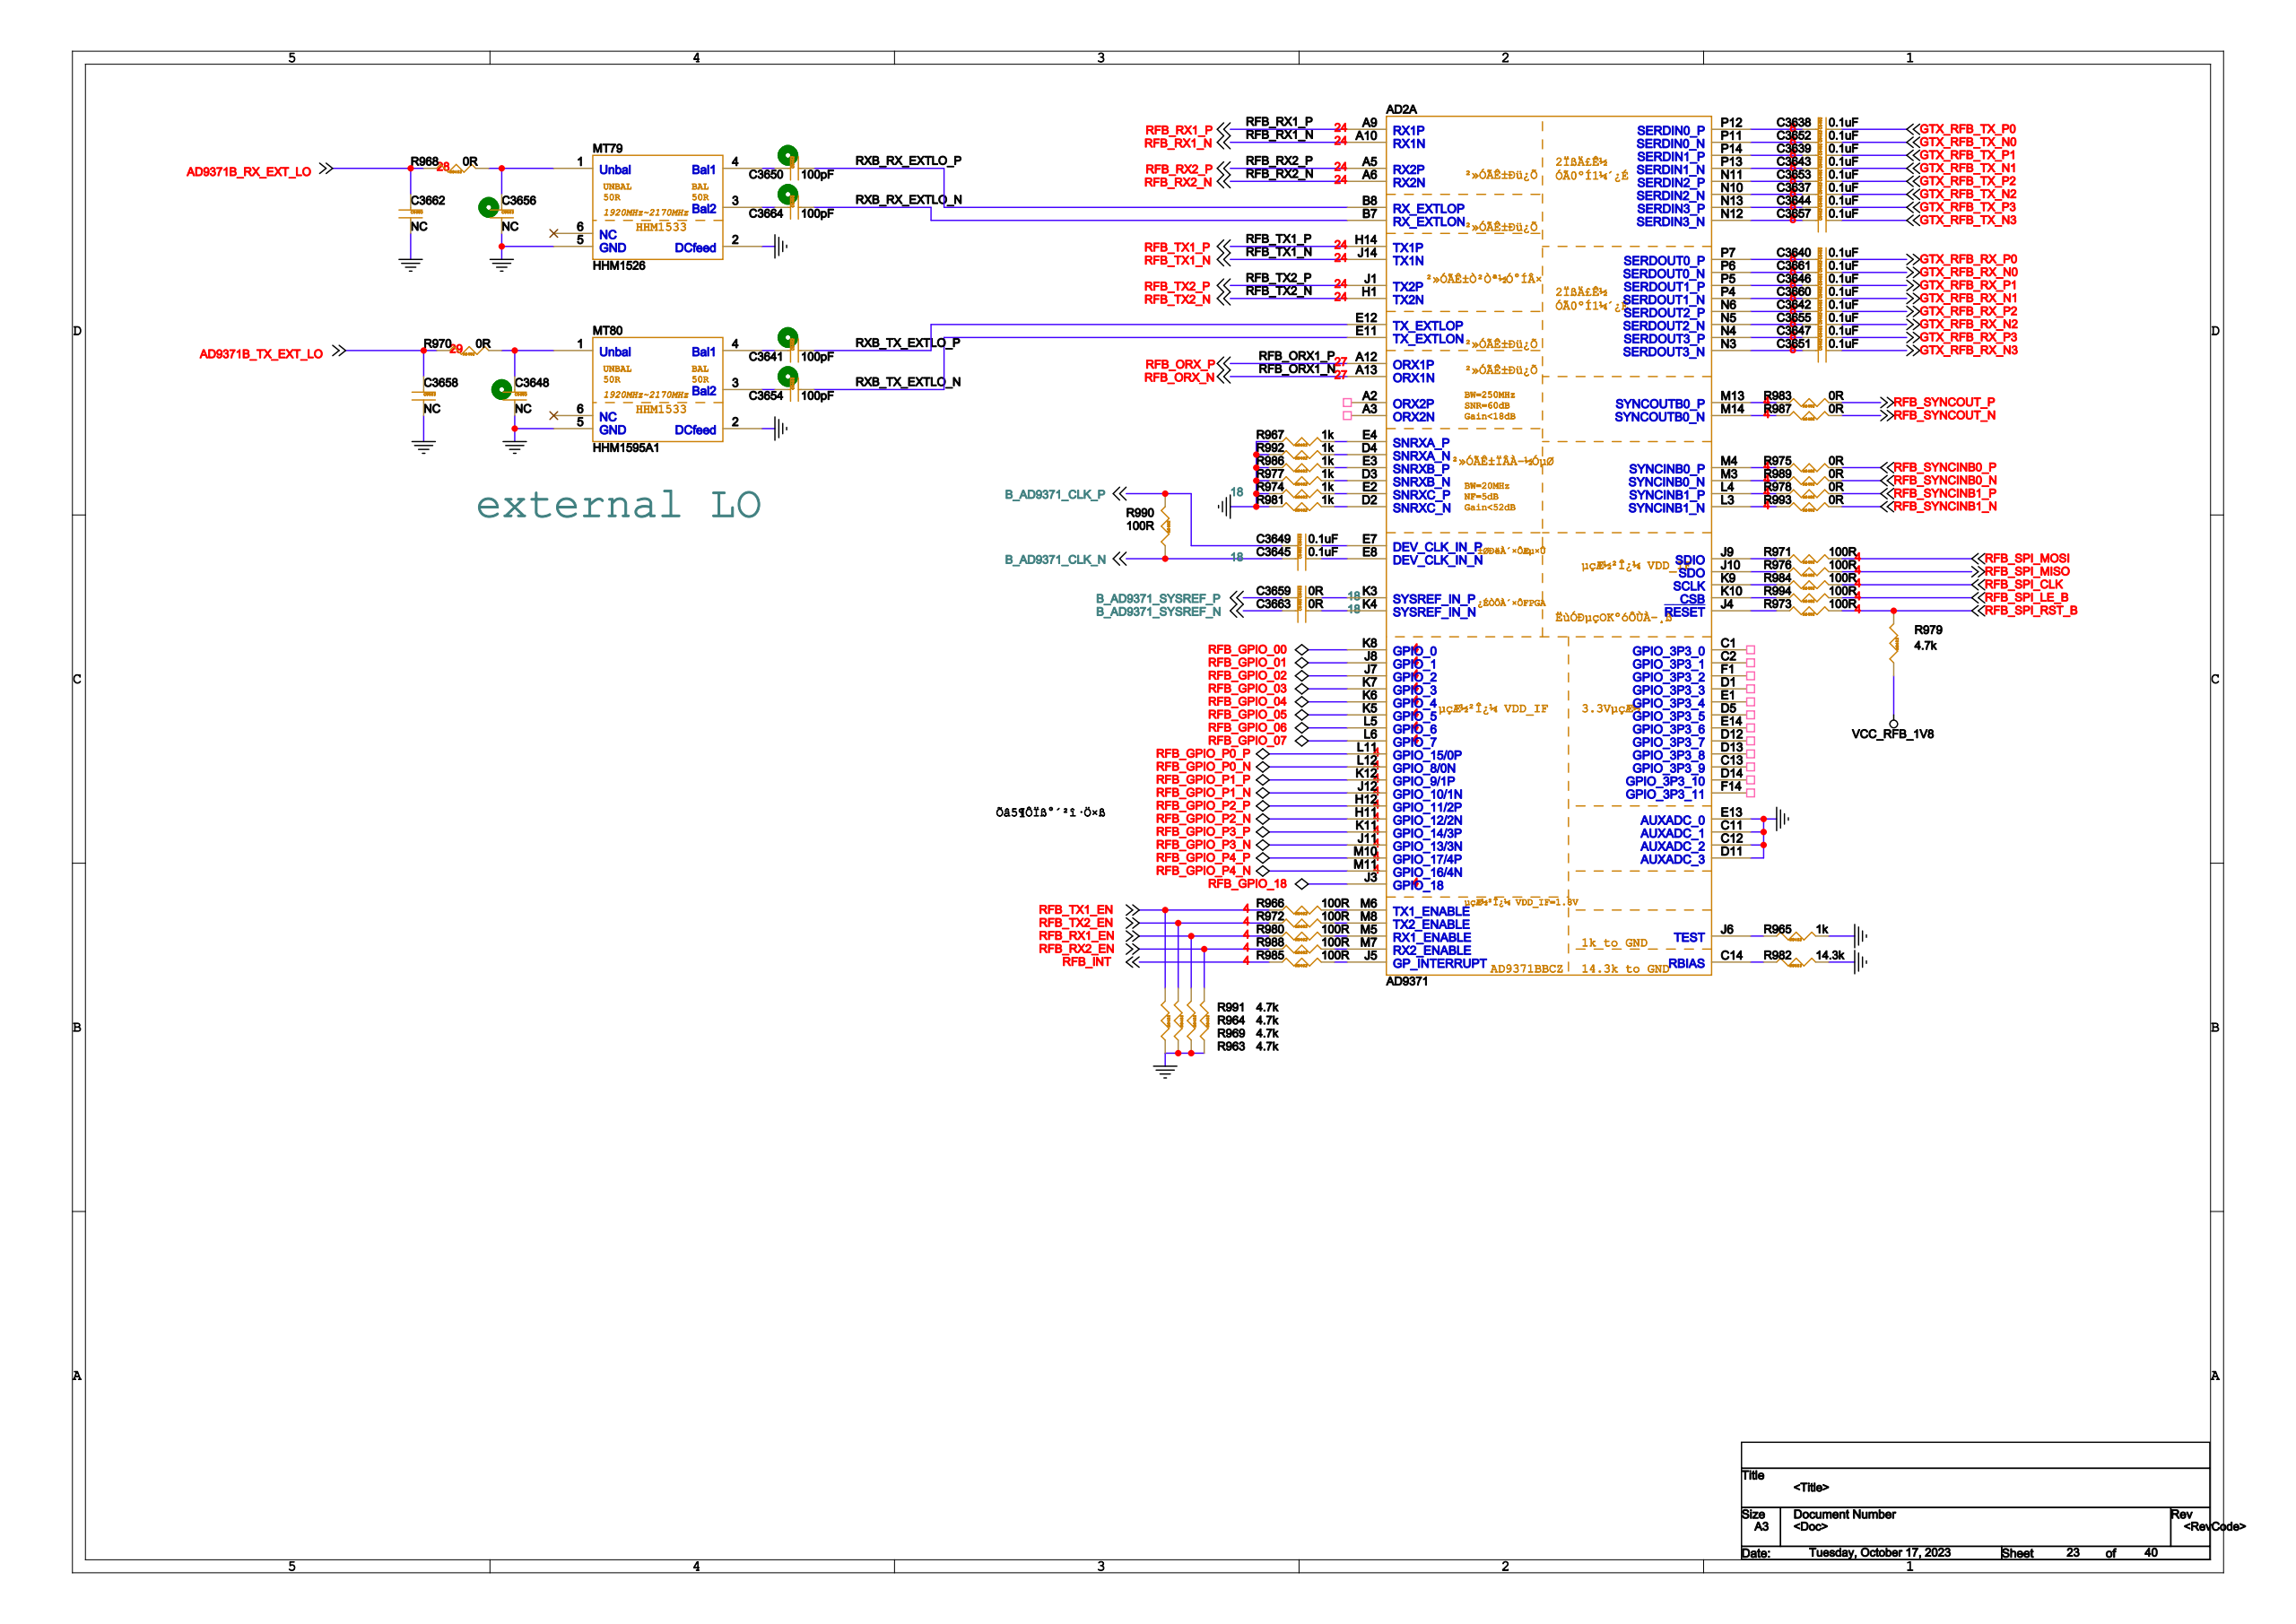Circuit board | Cadence Allegro | 1793 parts | 1223 nets | one sheet of the schematic
Parts on this sheet (reference | value | footprint):
AD2 | AD9371 | BGA196
C3637 | 0.1uF | C0402
C3638 | 0.1uF | C0402
C3639 | 0.1uF | C0402
C3640 | 0.1uF | C0402
C3641 | 100pF | C0402
C3642 | 0.1uF | C0402
C3643 | 0.1uF | C0402
C3644 | 0.1uF | C0402
C3645 | 0.1uF | C0402
C3646 | 0.1uF | C0402
C3647 | 0.1uF | C0402
C3648 | NC | C0402
C3649 | 0.1uF | C0402
C3650 | 100pF | C0402
C3651 | 0.1uF | C0402
C3652 | 0.1uF | C0402
C3653 | 0.1uF | C0402
C3654 | 100pF | C0402
C3655 | 0.1uF | C0402
C3656 | NC | C0402
C3657 | 0.1uF | C0402
C3658 | NC | C0402
C3659 | 0R | C0402
C3660 | 0.1uF | C0402
C3661 | 0.1uF | C0402
C3662 | NC | R0402
C3663 | 0R | C0402
C3664 | 100pF | C0402
MT79 | HHM1526 | HHM1595A1
MT80 | HHM1595A1 | HHM1595A1
R963 | 4.7k | R0402
R964 | 4.7k | R0402
R965 | 1k | R0402
R966 | 100R | R0402
R967 | 1k | R0402
R968 | 0R | R0402
R969 | 4.7k | R0402
R970 | 0R | R0402
R971 | 100R | R0402
R972 | 100R | R0402
R973 | 100R | R0402
R974 | 1k | R0402
R975 | 0R | R0402
R976 | 100R | R0402
R977 | 1k | R0402
R978 | 0R | R0402
R979 | 4.7k | R0402
R980 | 100R | R0402
R981 | 1k | R0402
R982 | 14.3k | R0402
R983 | 0R | R0402
R984 | 100R | R0402
R985 | 100R | R0402
R986 | 1k | R0402
R987 | 0R | R0402
R988 | 100R | R0402
R989 | 0R | R0402
R990 | 100R | R0402
R991 | 4.7k | R0402
R992 | 1k | R0402
R993 | 0R | R0402
R994 | 100R | R0402
Nets of these parts (net: part-pin ...):
GND: C3648-2 C3656-2 C3658-2 C3662-2 MT79-2 MT79-5 MT80-2 MT80-5 R963-1 R964-1 R965-2 R967-1 R969-1 R974-1 R977-1 R981-1 R982-2 R986-1 R991-1 R992-1 AD2-C11 AD2-C12 AD2-D11 AD2-E13
N17282126: C3650-1 MT79-4
N17282128: C3664-1 MT79-3
N17282120: C3656-1 MT79-1 R968-2
VCC_RFB_1V8: R979-1
N17282096: C3648-1 MT80-1 R970-2
AD9371B_TX_EXT_LO: C3658-1 R970-1
AD9371B_RX_EXT_LO: C3662-1 R968-1
N17282156: R994-1 AD2-K10
N17282216: C3645-2 AD2-E8
N17282214: C3649-2 AD2-E7
RFB_GPIO_00: AD2-K8
RFB_GPIO_01: AD2-J8
RFB_GPIO_P1_N: AD2-J12
RFB_GPIO_P2_P: AD2-H12
RFB_GPIO_P2_N: AD2-H11
RFB_GPIO_P3_N: AD2-J11
RFB_GPIO_P3_P: AD2-K11
RFB_GPIO_P0_P: AD2-L11
RFB_GPIO_P4_N: AD2-M11
RFB_GPIO_P4_P: AD2-M10
RFB_GPIO_18: AD2-J3
RFB_GPIO_02: AD2-J7
RFB_GPIO_03: AD2-K7
RFB_GPIO_04: AD2-K6
RFB_GPIO_05: AD2-K5
RFB_GPIO_06: AD2-L5
RFB_GPIO_07: AD2-L6
RFB_GPIO_P0_N: AD2-L12
RFB_GPIO_P1_P: AD2-K12
N18240491: R985-2 AD2-J5
RFB_ORX_N: AD2-A13
RFB_ORX_P: AD2-A12
N17282088: R982-1 AD2-C14
RFB_RX1_N: AD2-A10
RFB_RX1_P: AD2-A9
N18240490: R980-2 AD2-M5
RFB_RX2_N: AD2-A6
RFB_RX2_P: AD2-A5
N18240492: R988-2 AD2-M7
RXB_RX_EXTLO_N: C3664-2 AD2-B7
RXB_RX_EXTLO_P: C3650-2 AD2-B8
N17282158: R973-1 AD2-J4
N17282154: R984-1 AD2-K9
N17282150: R971-1 AD2-J9
N17282152: R976-1 AD2-J10
N17282014: C3652-1 AD2-P11
N17282012: C3638-1 AD2-P12
N17282018: C3643-1 AD2-P13
N17282016: C3639-1 AD2-P14
N17282022: C3637-1 AD2-N10
N17282020: C3653-1 AD2-N11
N17282026: C3657-1 AD2-N12
N17282024: C3644-1 AD2-N13
N17282200: C3661-1 AD2-P6
N17282198: C3640-1 AD2-P7
N17282204: C3660-1 AD2-P4
N17282202: C3646-1 AD2-P5
N17282208: C3655-1 AD2-N5
N17282206: C3642-1 AD2-N6
N17282212: C3651-1 AD2-N3
N17282210: C3647-1 AD2-N4
N17282038: R992-2 AD2-D4
N17282032: R967-2 AD2-E4
N17282050: R977-2 AD2-D3
N17282044: R986-2 AD2-E3
N17282062: R981-2 AD2-D2
N17282056: R974-2 AD2-E2
N18240438: R989-1 AD2-M3
N18240440: R975-1 AD2-M4
N18240437: R993-1 AD2-L3
N18240436: R978-1 AD2-L4
N18240435: R987-1 AD2-M14
N18240439: R983-1 AD2-M13
N17282066: C3663-2 AD2-K4
N17282064: C3659-2 AD2-K3
N17282084: R965-1 AD2-J6
RFB_TX1_N: AD2-J14
RFB_TX1_P: AD2-H14
N18240488: R966-2 AD2-M6
RFB_TX2_N: AD2-H1
RFB_TX2_P: AD2-J1
N18240489: R972-2 AD2-M8
RXB_TX_EXTLO_N: C3654-2 AD2-E11
RXB_TX_EXTLO_P: C3641-2 AD2-E12
GTX_RFB_TX_N2: C3637-2
GTX_RFB_TX_P0: C3638-2
GTX_RFB_TX_P1: C3639-2
GTX_RFB_RX_P0: C3640-2
GTX_RFB_RX_P2: C3642-2
GTX_RFB_TX_N1: C3643-2
GTX_RFB_TX_P3: C3644-2
B_AD9371_CLK_N: C3645-1 R990-1
GTX_RFB_RX_P1: C3646-2
GTX_RFB_RX_P3: C3647-2
B_AD9371_CLK_P: C3649-1 R990-2
GTX_RFB_RX_N3: C3651-2
GTX_RFB_TX_N0: C3652-2
GTX_RFB_TX_P2: C3653-2
GTX_RFB_RX_N2: C3655-2
GTX_RFB_TX_N3: C3657-2
GTX_RFB_RX_N1: C3660-2
GTX_RFB_RX_N0: C3661-2
B_AD9371_SYSREF_P: C3659-1
B_AD9371_SYSREF_N: C3663-1
N17282102: C3641-1 MT80-4
N17282104: C3654-1 MT80-3
RFB_SYNCINB0_P: R975-2
RFB_SYNCINB1_P: R978-2
RFB_SYNCOUT_P: R983-2
RFB_SYNCOUT_N: R987-2
RFB_SYNCINB0_N: R989-2
RFB_SYNCINB1_N: R993-2
RFB_TX1_EN: R966-1 R991-2
RFB_SPI_MOSI: R971-2
RFB_TX2_EN: R964-2 R972-1
RFB_SPI_RST_B: R973-2 R979-2
RFB_SPI_MISO: R976-2
RFB_RX1_EN: R969-2 R980-1
RFB_SPI_CLK: R984-2
RFB_INT: R985-1
RFB_RX2_EN: R963-2 R988-1
RFB_SPI_LE_B: R994-2